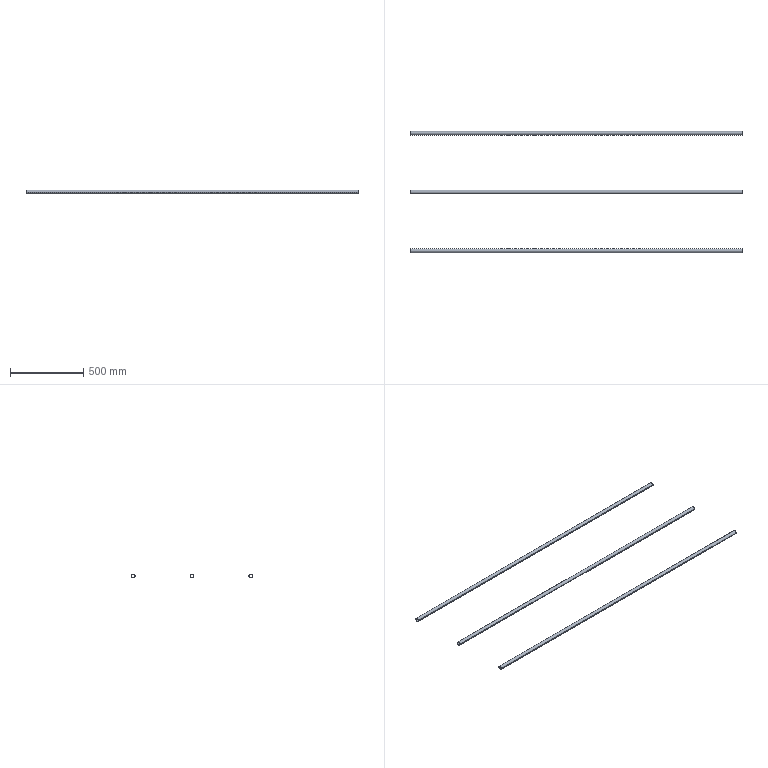Part | STEP file | E3-中转釜护栏8栏杆_Default<As Machined> | 3 solids | 18 faces | box 2260 x 825 x 25 mm | volume 750825 mm3 | cylinder 12 | plane 6 | commonest cylinder face diameters 22 x6 25 x6
STEP:
#1=CARTESIAN_POINT('',(0.,0.,0.));
#2=DIRECTION('',(0.,0.,1.));
#3=DIRECTION('',(1.,0.,0.));
#4=AXIS2_PLACEMENT_3D('',#1,#2,#3);
#5=CARTESIAN_POINT('',(1130.,787.5,0.));
#6=VERTEX_POINT('',#5);
#7=CARTESIAN_POINT('',(1130.,812.5,0.));
#8=VERTEX_POINT('',#7);
#9=CARTESIAN_POINT('',(1130.,800.,0.));
#10=DIRECTION('',(-1.,0.,0.));
#11=DIRECTION('',(0.,1.,0.));
#12=AXIS2_PLACEMENT_3D('',#9,#10,#11);
#13=CIRCLE('',#12,12.5);
#14=CARTESIAN_POINT('',(1130.,800.,0.));
#15=DIRECTION('',(-1.,0.,0.));
#16=DIRECTION('',(0.,-1.,0.));
#17=AXIS2_PLACEMENT_3D('',#14,#15,#16);
#18=CYLINDRICAL_SURFACE('',#17,12.5);
#19=CARTESIAN_POINT('',(-3.142,0.));
#20=DIRECTION('',(1.,0.));
#21=VECTOR('',#20,1.);
#22=LINE('',#19,#21);
#23=(GEOMETRIC_REPRESENTATION_CONTEXT(2)PARAMETRIC_REPRESENTATION_CONTEXT()REPRESENTATION_CONTEXT('',''));
#24=DEFINITIONAL_REPRESENTATION('',(#22),#23);
#25=PCURVE('',#18,#24);
#26=CARTESIAN_POINT('',(1130.,800.,0.));
#27=DIRECTION('',(1.,0.,0.));
#28=DIRECTION('',(0.,1.,0.));
#29=AXIS2_PLACEMENT_3D('',#26,#27,#28);
#30=PLANE('',#29);
#31=CARTESIAN_POINT('',(12.5,0.));
#32=CARTESIAN_POINT('',(12.5,-21.651));
#33=CARTESIAN_POINT('',(-6.25,-10.825));
#34=CARTESIAN_POINT('',(-25.,0.));
#35=CARTESIAN_POINT('',(-6.25,10.825));
#36=CARTESIAN_POINT('',(12.5,21.651));
#37=CARTESIAN_POINT('',(12.5,0.));
#38=(BOUNDED_CURVE()B_SPLINE_CURVE(2,(#31,#32,#33,#34,#35,#36,#37),.UNSPECIFIED.,.T.,.F.)B_SPLINE_CURVE_WITH_KNOTS((1,2,2,2,2,1),(-2.094,0.,2.094,4.189,6.283,8.378),.UNSPECIFIED.)CURVE()GEOMETRIC_REPRESENTATION_ITEM()RATIONAL_B_SPLINE_CURVE((1.,0.5,1.,0.5,1.,0.5,1.))REPRESENTATION_ITEM(''));
#39=(GEOMETRIC_REPRESENTATION_CONTEXT(2)PARAMETRIC_REPRESENTATION_CONTEXT()REPRESENTATION_CONTEXT('',''));
#40=DEFINITIONAL_REPRESENTATION('',(#38),#39);
#41=PCURVE('',#30,#40);
#42=SURFACE_CURVE('',#13,(#25,#41),.PCURVE_S1.);
#43=EDGE_CURVE('',#6,#8,#42,.T.);
#44=ORIENTED_EDGE('',*,*,#43,.T.);
#45=CARTESIAN_POINT('',(-1130.,812.5,0.));
#46=VERTEX_POINT('',#45);
#47=CARTESIAN_POINT('',(1130.,812.5,0.));
#48=DIRECTION('',(-1.,0.,0.));
#49=VECTOR('',#48,1.);
#50=LINE('',#47,#49);
#51=CARTESIAN_POINT('',(3.142,0.));
#52=DIRECTION('',(0.,1.));
#53=VECTOR('',#52,1.);
#54=LINE('',#51,#53);
#55=(GEOMETRIC_REPRESENTATION_CONTEXT(2)PARAMETRIC_REPRESENTATION_CONTEXT()REPRESENTATION_CONTEXT('',''));
#56=DEFINITIONAL_REPRESENTATION('',(#54),#55);
#57=PCURVE('',#18,#56);
#58=CARTESIAN_POINT('',(1130.,800.,0.));
#59=DIRECTION('',(-1.,0.,0.));
#60=DIRECTION('',(0.,-1.,0.));
#61=AXIS2_PLACEMENT_3D('',#58,#59,#60);
#62=CYLINDRICAL_SURFACE('',#61,12.5);
#63=CARTESIAN_POINT('',(3.142,0.));
#64=DIRECTION('',(0.,1.));
#65=VECTOR('',#64,1.);
#66=LINE('',#63,#65);
#67=(GEOMETRIC_REPRESENTATION_CONTEXT(2)PARAMETRIC_REPRESENTATION_CONTEXT()REPRESENTATION_CONTEXT('',''));
#68=DEFINITIONAL_REPRESENTATION('',(#66),#67);
#69=PCURVE('',#62,#68);
#70=SURFACE_CURVE('',#50,(#57,#69),.PCURVE_S1.);
#71=EDGE_CURVE('',#8,#46,#70,.T.);
#72=ORIENTED_EDGE('',*,*,#71,.T.);
#73=CARTESIAN_POINT('',(-1130.,787.5,0.));
#74=VERTEX_POINT('',#73);
#75=CARTESIAN_POINT('',(-1130.,800.,0.));
#76=DIRECTION('',(-1.,0.,0.));
#77=DIRECTION('',(0.,1.,0.));
#78=AXIS2_PLACEMENT_3D('',#75,#76,#77);
#79=CIRCLE('',#78,12.5);
#80=CARTESIAN_POINT('',(-3.142,2260.));
#81=DIRECTION('',(1.,0.));
#82=VECTOR('',#81,1.);
#83=LINE('',#80,#82);
#84=(GEOMETRIC_REPRESENTATION_CONTEXT(2)PARAMETRIC_REPRESENTATION_CONTEXT()REPRESENTATION_CONTEXT('',''));
#85=DEFINITIONAL_REPRESENTATION('',(#83),#84);
#86=PCURVE('',#18,#85);
#87=CARTESIAN_POINT('',(-1130.,800.,0.));
#88=DIRECTION('',(1.,0.,0.));
#89=DIRECTION('',(0.,1.,0.));
#90=AXIS2_PLACEMENT_3D('',#87,#88,#89);
#91=PLANE('',#90);
#92=CARTESIAN_POINT('',(12.5,0.));
#93=CARTESIAN_POINT('',(12.5,-21.651));
#94=CARTESIAN_POINT('',(-6.25,-10.825));
#95=CARTESIAN_POINT('',(-25.,0.));
#96=CARTESIAN_POINT('',(-6.25,10.825));
#97=CARTESIAN_POINT('',(12.5,21.651));
#98=CARTESIAN_POINT('',(12.5,0.));
#99=(BOUNDED_CURVE()B_SPLINE_CURVE(2,(#92,#93,#94,#95,#96,#97,#98),.UNSPECIFIED.,.T.,.F.)B_SPLINE_CURVE_WITH_KNOTS((1,2,2,2,2,1),(-2.094,0.,2.094,4.189,6.283,8.378),.UNSPECIFIED.)CURVE()GEOMETRIC_REPRESENTATION_ITEM()RATIONAL_B_SPLINE_CURVE((1.,0.5,1.,0.5,1.,0.5,1.))REPRESENTATION_ITEM(''));
#100=(GEOMETRIC_REPRESENTATION_CONTEXT(2)PARAMETRIC_REPRESENTATION_CONTEXT()REPRESENTATION_CONTEXT('',''));
#101=DEFINITIONAL_REPRESENTATION('',(#99),#100);
#102=PCURVE('',#91,#101);
#103=SURFACE_CURVE('',#79,(#86,#102),.PCURVE_S1.);
#104=EDGE_CURVE('',#74,#46,#103,.T.);
#105=ORIENTED_EDGE('',*,*,#104,.F.);
#106=CARTESIAN_POINT('',(1130.,787.5,0.));
#107=DIRECTION('',(-1.,0.,0.));
#108=VECTOR('',#107,1.);
#109=LINE('',#106,#108);
#110=CARTESIAN_POINT('',(0.,0.));
#111=DIRECTION('',(0.,1.));
#112=VECTOR('',#111,1.);
#113=LINE('',#110,#112);
#114=(GEOMETRIC_REPRESENTATION_CONTEXT(2)PARAMETRIC_REPRESENTATION_CONTEXT()REPRESENTATION_CONTEXT('',''));
#115=DEFINITIONAL_REPRESENTATION('',(#113),#114);
#116=PCURVE('',#18,#115);
#117=CARTESIAN_POINT('',(6.283,0.));
#118=DIRECTION('',(0.,1.));
#119=VECTOR('',#118,1.);
#120=LINE('',#117,#119);
#121=(GEOMETRIC_REPRESENTATION_CONTEXT(2)PARAMETRIC_REPRESENTATION_CONTEXT()REPRESENTATION_CONTEXT('',''));
#122=DEFINITIONAL_REPRESENTATION('',(#120),#121);
#123=PCURVE('',#62,#122);
#124=SURFACE_CURVE('',#109,(#116,#123),.PCURVE_S1.);
#125=EDGE_CURVE('',#6,#74,#124,.T.);
#126=ORIENTED_EDGE('',*,*,#125,.F.);
#127=EDGE_LOOP('',(#44,#72,#105,#126));
#128=FACE_BOUND('',#127,.T.);
#129=ADVANCED_FACE('',(#128),#18,.T.);
#130=CARTESIAN_POINT('',(1130.,789.,0.));
#131=VERTEX_POINT('',#130);
#132=CARTESIAN_POINT('',(-1130.,789.,0.));
#133=VERTEX_POINT('',#132);
#134=CARTESIAN_POINT('',(1130.,789.,0.));
#135=DIRECTION('',(-1.,0.,0.));
#136=VECTOR('',#135,1.);
#137=LINE('',#134,#136);
#138=CARTESIAN_POINT('',(1130.,800.,0.));
#139=DIRECTION('',(-1.,0.,0.));
#140=DIRECTION('',(0.,-1.,0.));
#141=AXIS2_PLACEMENT_3D('',#138,#139,#140);
#142=CYLINDRICAL_SURFACE('',#141,11.);
#143=CARTESIAN_POINT('',(6.283,0.));
#144=DIRECTION('',(0.,1.));
#145=VECTOR('',#144,1.);
#146=LINE('',#143,#145);
#147=(GEOMETRIC_REPRESENTATION_CONTEXT(2)PARAMETRIC_REPRESENTATION_CONTEXT()REPRESENTATION_CONTEXT('',''));
#148=DEFINITIONAL_REPRESENTATION('',(#146),#147);
#149=PCURVE('',#142,#148);
#150=CARTESIAN_POINT('',(1130.,800.,0.));
#151=DIRECTION('',(-1.,0.,0.));
#152=DIRECTION('',(0.,-1.,0.));
#153=AXIS2_PLACEMENT_3D('',#150,#151,#152);
#154=CYLINDRICAL_SURFACE('',#153,11.);
#155=CARTESIAN_POINT('',(0.,0.));
#156=DIRECTION('',(0.,1.));
#157=VECTOR('',#156,1.);
#158=LINE('',#155,#157);
#159=(GEOMETRIC_REPRESENTATION_CONTEXT(2)PARAMETRIC_REPRESENTATION_CONTEXT()REPRESENTATION_CONTEXT('',''));
#160=DEFINITIONAL_REPRESENTATION('',(#158),#159);
#161=PCURVE('',#154,#160);
#162=SURFACE_CURVE('',#137,(#149,#161),.PCURVE_S1.);
#163=EDGE_CURVE('',#131,#133,#162,.T.);
#164=ORIENTED_EDGE('',*,*,#163,.T.);
#165=CARTESIAN_POINT('',(-1130.,811.,0.));
#166=VERTEX_POINT('',#165);
#167=CARTESIAN_POINT('',(-1130.,800.,0.));
#168=DIRECTION('',(-1.,0.,0.));
#169=DIRECTION('',(0.,1.,0.));
#170=AXIS2_PLACEMENT_3D('',#167,#168,#169);
#171=CIRCLE('',#170,11.);
#172=CARTESIAN_POINT('',(3.142,2260.));
#173=DIRECTION('',(1.,0.));
#174=VECTOR('',#173,1.);
#175=LINE('',#172,#174);
#176=(GEOMETRIC_REPRESENTATION_CONTEXT(2)PARAMETRIC_REPRESENTATION_CONTEXT()REPRESENTATION_CONTEXT('',''));
#177=DEFINITIONAL_REPRESENTATION('',(#175),#176);
#178=PCURVE('',#142,#177);
#179=CARTESIAN_POINT('',(11.,0.));
#180=CARTESIAN_POINT('',(11.,-19.053));
#181=CARTESIAN_POINT('',(-5.5,-9.526));
#182=CARTESIAN_POINT('',(-22.,0.));
#183=CARTESIAN_POINT('',(-5.5,9.526));
#184=CARTESIAN_POINT('',(11.,19.053));
#185=CARTESIAN_POINT('',(11.,0.));
#186=(BOUNDED_CURVE()B_SPLINE_CURVE(2,(#179,#180,#181,#182,#183,#184,#185),.UNSPECIFIED.,.T.,.F.)B_SPLINE_CURVE_WITH_KNOTS((1,2,2,2,2,1),(-2.094,0.,2.094,4.189,6.283,8.378),.UNSPECIFIED.)CURVE()GEOMETRIC_REPRESENTATION_ITEM()RATIONAL_B_SPLINE_CURVE((1.,0.5,1.,0.5,1.,0.5,1.))REPRESENTATION_ITEM(''));
#187=(GEOMETRIC_REPRESENTATION_CONTEXT(2)PARAMETRIC_REPRESENTATION_CONTEXT()REPRESENTATION_CONTEXT('',''));
#188=DEFINITIONAL_REPRESENTATION('',(#186),#187);
#189=PCURVE('',#91,#188);
#190=SURFACE_CURVE('',#171,(#178,#189),.PCURVE_S1.);
#191=EDGE_CURVE('',#166,#133,#190,.T.);
#192=ORIENTED_EDGE('',*,*,#191,.F.);
#193=CARTESIAN_POINT('',(1130.,811.,0.));
#194=VERTEX_POINT('',#193);
#195=CARTESIAN_POINT('',(1130.,811.,0.));
#196=DIRECTION('',(-1.,0.,0.));
#197=VECTOR('',#196,1.);
#198=LINE('',#195,#197);
#199=CARTESIAN_POINT('',(3.142,0.));
#200=DIRECTION('',(0.,1.));
#201=VECTOR('',#200,1.);
#202=LINE('',#199,#201);
#203=(GEOMETRIC_REPRESENTATION_CONTEXT(2)PARAMETRIC_REPRESENTATION_CONTEXT()REPRESENTATION_CONTEXT('',''));
#204=DEFINITIONAL_REPRESENTATION('',(#202),#203);
#205=PCURVE('',#142,#204);
#206=CARTESIAN_POINT('',(3.142,0.));
#207=DIRECTION('',(0.,1.));
#208=VECTOR('',#207,1.);
#209=LINE('',#206,#208);
#210=(GEOMETRIC_REPRESENTATION_CONTEXT(2)PARAMETRIC_REPRESENTATION_CONTEXT()REPRESENTATION_CONTEXT('',''));
#211=DEFINITIONAL_REPRESENTATION('',(#209),#210);
#212=PCURVE('',#154,#211);
#213=SURFACE_CURVE('',#198,(#205,#212),.PCURVE_S1.);
#214=EDGE_CURVE('',#194,#166,#213,.T.);
#215=ORIENTED_EDGE('',*,*,#214,.F.);
#216=CARTESIAN_POINT('',(1130.,800.,0.));
#217=DIRECTION('',(-1.,0.,0.));
#218=DIRECTION('',(0.,1.,0.));
#219=AXIS2_PLACEMENT_3D('',#216,#217,#218);
#220=CIRCLE('',#219,11.);
#221=CARTESIAN_POINT('',(3.142,0.));
#222=DIRECTION('',(1.,0.));
#223=VECTOR('',#222,1.);
#224=LINE('',#221,#223);
#225=(GEOMETRIC_REPRESENTATION_CONTEXT(2)PARAMETRIC_REPRESENTATION_CONTEXT()REPRESENTATION_CONTEXT('',''));
#226=DEFINITIONAL_REPRESENTATION('',(#224),#225);
#227=PCURVE('',#142,#226);
#228=CARTESIAN_POINT('',(11.,0.));
#229=CARTESIAN_POINT('',(11.,-19.053));
#230=CARTESIAN_POINT('',(-5.5,-9.526));
#231=CARTESIAN_POINT('',(-22.,0.));
#232=CARTESIAN_POINT('',(-5.5,9.526));
#233=CARTESIAN_POINT('',(11.,19.053));
#234=CARTESIAN_POINT('',(11.,0.));
#235=(BOUNDED_CURVE()B_SPLINE_CURVE(2,(#228,#229,#230,#231,#232,#233,#234),.UNSPECIFIED.,.T.,.F.)B_SPLINE_CURVE_WITH_KNOTS((1,2,2,2,2,1),(-2.094,0.,2.094,4.189,6.283,8.378),.UNSPECIFIED.)CURVE()GEOMETRIC_REPRESENTATION_ITEM()RATIONAL_B_SPLINE_CURVE((1.,0.5,1.,0.5,1.,0.5,1.))REPRESENTATION_ITEM(''));
#236=(GEOMETRIC_REPRESENTATION_CONTEXT(2)PARAMETRIC_REPRESENTATION_CONTEXT()REPRESENTATION_CONTEXT('',''));
#237=DEFINITIONAL_REPRESENTATION('',(#235),#236);
#238=PCURVE('',#30,#237);
#239=SURFACE_CURVE('',#220,(#227,#238),.PCURVE_S1.);
#240=EDGE_CURVE('',#194,#131,#239,.T.);
#241=ORIENTED_EDGE('',*,*,#240,.T.);
#242=EDGE_LOOP('',(#164,#192,#215,#241));
#243=FACE_BOUND('',#242,.F.);
#244=ADVANCED_FACE('',(#243),#142,.F.);
#245=CARTESIAN_POINT('',(-1130.,800.,0.));
#246=DIRECTION('',(-1.,0.,0.));
#247=DIRECTION('',(0.,1.,0.));
#248=AXIS2_PLACEMENT_3D('',#245,#246,#247);
#249=CIRCLE('',#248,11.);
#250=CARTESIAN_POINT('',(-3.142,2260.));
#251=DIRECTION('',(1.,0.));
#252=VECTOR('',#251,1.);
#253=LINE('',#250,#252);
#254=(GEOMETRIC_REPRESENTATION_CONTEXT(2)PARAMETRIC_REPRESENTATION_CONTEXT()REPRESENTATION_CONTEXT('',''));
#255=DEFINITIONAL_REPRESENTATION('',(#253),#254);
#256=PCURVE('',#154,#255);
#257=CARTESIAN_POINT('',(11.,0.));
#258=CARTESIAN_POINT('',(11.,-19.053));
#259=CARTESIAN_POINT('',(-5.5,-9.526));
#260=CARTESIAN_POINT('',(-22.,0.));
#261=CARTESIAN_POINT('',(-5.5,9.526));
#262=CARTESIAN_POINT('',(11.,19.053));
#263=CARTESIAN_POINT('',(11.,0.));
#264=(BOUNDED_CURVE()B_SPLINE_CURVE(2,(#257,#258,#259,#260,#261,#262,#263),.UNSPECIFIED.,.T.,.F.)B_SPLINE_CURVE_WITH_KNOTS((1,2,2,2,2,1),(-2.094,0.,2.094,4.189,6.283,8.378),.UNSPECIFIED.)CURVE()GEOMETRIC_REPRESENTATION_ITEM()RATIONAL_B_SPLINE_CURVE((1.,0.5,1.,0.5,1.,0.5,1.))REPRESENTATION_ITEM(''));
#265=(GEOMETRIC_REPRESENTATION_CONTEXT(2)PARAMETRIC_REPRESENTATION_CONTEXT()REPRESENTATION_CONTEXT('',''));
#266=DEFINITIONAL_REPRESENTATION('',(#264),#265);
#267=PCURVE('',#91,#266);
#268=SURFACE_CURVE('',#249,(#256,#267),.PCURVE_S1.);
#269=EDGE_CURVE('',#133,#166,#268,.T.);
#270=ORIENTED_EDGE('',*,*,#269,.F.);
#271=ORIENTED_EDGE('',*,*,#163,.F.);
#272=CARTESIAN_POINT('',(1130.,800.,0.));
#273=DIRECTION('',(-1.,0.,0.));
#274=DIRECTION('',(0.,1.,0.));
#275=AXIS2_PLACEMENT_3D('',#272,#273,#274);
#276=CIRCLE('',#275,11.);
#277=CARTESIAN_POINT('',(-3.142,0.));
#278=DIRECTION('',(1.,0.));
#279=VECTOR('',#278,1.);
#280=LINE('',#277,#279);
#281=(GEOMETRIC_REPRESENTATION_CONTEXT(2)PARAMETRIC_REPRESENTATION_CONTEXT()REPRESENTATION_CONTEXT('',''));
#282=DEFINITIONAL_REPRESENTATION('',(#280),#281);
#283=PCURVE('',#154,#282);
#284=CARTESIAN_POINT('',(11.,0.));
#285=CARTESIAN_POINT('',(11.,-19.053));
#286=CARTESIAN_POINT('',(-5.5,-9.526));
#287=CARTESIAN_POINT('',(-22.,0.));
#288=CARTESIAN_POINT('',(-5.5,9.526));
#289=CARTESIAN_POINT('',(11.,19.053));
#290=CARTESIAN_POINT('',(11.,0.));
#291=(BOUNDED_CURVE()B_SPLINE_CURVE(2,(#284,#285,#286,#287,#288,#289,#290),.UNSPECIFIED.,.T.,.F.)B_SPLINE_CURVE_WITH_KNOTS((1,2,2,2,2,1),(-2.094,0.,2.094,4.189,6.283,8.378),.UNSPECIFIED.)CURVE()GEOMETRIC_REPRESENTATION_ITEM()RATIONAL_B_SPLINE_CURVE((1.,0.5,1.,0.5,1.,0.5,1.))REPRESENTATION_ITEM(''));
#292=(GEOMETRIC_REPRESENTATION_CONTEXT(2)PARAMETRIC_REPRESENTATION_CONTEXT()REPRESENTATION_CONTEXT('',''));
#293=DEFINITIONAL_REPRESENTATION('',(#291),#292);
#294=PCURVE('',#30,#293);
#295=SURFACE_CURVE('',#276,(#283,#294),.PCURVE_S1.);
#296=EDGE_CURVE('',#131,#194,#295,.T.);
#297=ORIENTED_EDGE('',*,*,#296,.T.);
#298=ORIENTED_EDGE('',*,*,#214,.T.);
#299=EDGE_LOOP('',(#270,#271,#297,#298));
#300=FACE_BOUND('',#299,.F.);
#301=ADVANCED_FACE('',(#300),#154,.F.);
#302=ORIENTED_EDGE('',*,*,#71,.F.);
#303=CARTESIAN_POINT('',(1130.,800.,0.));
#304=DIRECTION('',(-1.,0.,0.));
#305=DIRECTION('',(0.,1.,0.));
#306=AXIS2_PLACEMENT_3D('',#303,#304,#305);
#307=CIRCLE('',#306,12.5);
#308=CARTESIAN_POINT('',(3.142,0.));
#309=DIRECTION('',(1.,0.));
#310=VECTOR('',#309,1.);
#311=LINE('',#308,#310);
#312=(GEOMETRIC_REPRESENTATION_CONTEXT(2)PARAMETRIC_REPRESENTATION_CONTEXT()REPRESENTATION_CONTEXT('',''));
#313=DEFINITIONAL_REPRESENTATION('',(#311),#312);
#314=PCURVE('',#62,#313);
#315=CARTESIAN_POINT('',(12.5,0.));
#316=CARTESIAN_POINT('',(12.5,-21.651));
#317=CARTESIAN_POINT('',(-6.25,-10.825));
#318=CARTESIAN_POINT('',(-25.,0.));
#319=CARTESIAN_POINT('',(-6.25,10.825));
#320=CARTESIAN_POINT('',(12.5,21.651));
#321=CARTESIAN_POINT('',(12.5,0.));
#322=(BOUNDED_CURVE()B_SPLINE_CURVE(2,(#315,#316,#317,#318,#319,#320,#321),.UNSPECIFIED.,.T.,.F.)B_SPLINE_CURVE_WITH_KNOTS((1,2,2,2,2,1),(-2.094,0.,2.094,4.189,6.283,8.378),.UNSPECIFIED.)CURVE()GEOMETRIC_REPRESENTATION_ITEM()RATIONAL_B_SPLINE_CURVE((1.,0.5,1.,0.5,1.,0.5,1.))REPRESENTATION_ITEM(''));
#323=(GEOMETRIC_REPRESENTATION_CONTEXT(2)PARAMETRIC_REPRESENTATION_CONTEXT()REPRESENTATION_CONTEXT('',''));
#324=DEFINITIONAL_REPRESENTATION('',(#322),#323);
#325=PCURVE('',#30,#324);
#326=SURFACE_CURVE('',#307,(#314,#325),.PCURVE_S1.);
#327=EDGE_CURVE('',#8,#6,#326,.T.);
#328=ORIENTED_EDGE('',*,*,#327,.T.);
#329=ORIENTED_EDGE('',*,*,#125,.T.);
#330=CARTESIAN_POINT('',(-1130.,800.,0.));
#331=DIRECTION('',(-1.,0.,0.));
#332=DIRECTION('',(0.,1.,0.));
#333=AXIS2_PLACEMENT_3D('',#330,#331,#332);
#334=CIRCLE('',#333,12.5);
#335=CARTESIAN_POINT('',(3.142,2260.));
#336=DIRECTION('',(1.,0.));
#337=VECTOR('',#336,1.);
#338=LINE('',#335,#337);
#339=(GEOMETRIC_REPRESENTATION_CONTEXT(2)PARAMETRIC_REPRESENTATION_CONTEXT()REPRESENTATION_CONTEXT('',''));
#340=DEFINITIONAL_REPRESENTATION('',(#338),#339);
#341=PCURVE('',#62,#340);
#342=CARTESIAN_POINT('',(12.5,0.));
#343=CARTESIAN_POINT('',(12.5,-21.651));
#344=CARTESIAN_POINT('',(-6.25,-10.825));
#345=CARTESIAN_POINT('',(-25.,0.));
#346=CARTESIAN_POINT('',(-6.25,10.825));
#347=CARTESIAN_POINT('',(12.5,21.651));
#348=CARTESIAN_POINT('',(12.5,0.));
#349=(BOUNDED_CURVE()B_SPLINE_CURVE(2,(#342,#343,#344,#345,#346,#347,#348),.UNSPECIFIED.,.T.,.F.)B_SPLINE_CURVE_WITH_KNOTS((1,2,2,2,2,1),(-2.094,0.,2.094,4.189,6.283,8.378),.UNSPECIFIED.)CURVE()GEOMETRIC_REPRESENTATION_ITEM()RATIONAL_B_SPLINE_CURVE((1.,0.5,1.,0.5,1.,0.5,1.))REPRESENTATION_ITEM(''));
#350=(GEOMETRIC_REPRESENTATION_CONTEXT(2)PARAMETRIC_REPRESENTATION_CONTEXT()REPRESENTATION_CONTEXT('',''));
#351=DEFINITIONAL_REPRESENTATION('',(#349),#350);
#352=PCURVE('',#91,#351);
#353=SURFACE_CURVE('',#334,(#341,#352),.PCURVE_S1.);
#354=EDGE_CURVE('',#46,#74,#353,.T.);
#355=ORIENTED_EDGE('',*,*,#354,.F.);
#356=EDGE_LOOP('',(#302,#328,#329,#355));
#357=FACE_BOUND('',#356,.T.);
#358=ADVANCED_FACE('',(#357),#62,.T.);
#359=ORIENTED_EDGE('',*,*,#296,.T.);
#360=ORIENTED_EDGE('',*,*,#240,.T.);
#361=EDGE_LOOP('',(#359,#360));
#362=FACE_BOUND('',#361,.T.);
#363=ORIENTED_EDGE('',*,*,#43,.F.);
#364=ORIENTED_EDGE('',*,*,#327,.F.);
#365=EDGE_LOOP('',(#363,#364));
#366=FACE_BOUND('',#365,.T.);
#367=ADVANCED_FACE('',(#362,#366),#30,.T.);
#368=ORIENTED_EDGE('',*,*,#269,.F.);
#369=ORIENTED_EDGE('',*,*,#191,.F.);
#370=EDGE_LOOP('',(#368,#369));
#371=FACE_BOUND('',#370,.T.);
#372=ORIENTED_EDGE('',*,*,#104,.T.);
#373=ORIENTED_EDGE('',*,*,#354,.T.);
#374=EDGE_LOOP('',(#372,#373));
#375=FACE_BOUND('',#374,.T.);
#376=ADVANCED_FACE('',(#371,#375),#91,.F.);
#377=CLOSED_SHELL('',(#129,#244,#301,#358,#367,#376));
#378=MANIFOLD_SOLID_BREP('',#377);
#379=CARTESIAN_POINT('',(1130.,-12.5,0.));
#380=VERTEX_POINT('',#379);
#381=CARTESIAN_POINT('',(1130.,12.5,0.));
#382=VERTEX_POINT('',#381);
#383=CARTESIAN_POINT('',(1130.,0.,0.));
#384=DIRECTION('',(-1.,0.,0.));
#385=DIRECTION('',(0.,1.,0.));
#386=AXIS2_PLACEMENT_3D('',#383,#384,#385);
#387=CIRCLE('',#386,12.5);
#388=CARTESIAN_POINT('',(1130.,0.,0.));
#389=DIRECTION('',(-1.,0.,0.));
#390=DIRECTION('',(0.,-1.,0.));
#391=AXIS2_PLACEMENT_3D('',#388,#389,#390);
#392=CYLINDRICAL_SURFACE('',#391,12.5);
#393=CARTESIAN_POINT('',(-3.142,0.));
#394=DIRECTION('',(1.,0.));
#395=VECTOR('',#394,1.);
#396=LINE('',#393,#395);
#397=(GEOMETRIC_REPRESENTATION_CONTEXT(2)PARAMETRIC_REPRESENTATION_CONTEXT()REPRESENTATION_CONTEXT('',''));
#398=DEFINITIONAL_REPRESENTATION('',(#396),#397);
#399=PCURVE('',#392,#398);
#400=CARTESIAN_POINT('',(1130.,0.,0.));
#401=DIRECTION('',(1.,0.,0.));
#402=DIRECTION('',(0.,1.,0.));
#403=AXIS2_PLACEMENT_3D('',#400,#401,#402);
#404=PLANE('',#403);
#405=CARTESIAN_POINT('',(12.5,0.));
#406=CARTESIAN_POINT('',(12.5,-21.651));
#407=CARTESIAN_POINT('',(-6.25,-10.825));
#408=CARTESIAN_POINT('',(-25.,0.));
#409=CARTESIAN_POINT('',(-6.25,10.825));
#410=CARTESIAN_POINT('',(12.5,21.651));
#411=CARTESIAN_POINT('',(12.5,0.));
#412=(BOUNDED_CURVE()B_SPLINE_CURVE(2,(#405,#406,#407,#408,#409,#410,#411),.UNSPECIFIED.,.T.,.F.)B_SPLINE_CURVE_WITH_KNOTS((1,2,2,2,2,1),(-2.094,0.,2.094,4.189,6.283,8.378),.UNSPECIFIED.)CURVE()GEOMETRIC_REPRESENTATION_ITEM()RATIONAL_B_SPLINE_CURVE((1.,0.5,1.,0.5,1.,0.5,1.))REPRESENTATION_ITEM(''));
#413=(GEOMETRIC_REPRESENTATION_CONTEXT(2)PARAMETRIC_REPRESENTATION_CONTEXT()REPRESENTATION_CONTEXT('',''));
#414=DEFINITIONAL_REPRESENTATION('',(#412),#413);
#415=PCURVE('',#404,#414);
#416=SURFACE_CURVE('',#387,(#399,#415),.PCURVE_S1.);
#417=EDGE_CURVE('',#380,#382,#416,.T.);
#418=ORIENTED_EDGE('',*,*,#417,.T.);
#419=CARTESIAN_POINT('',(-1130.,12.5,0.));
#420=VERTEX_POINT('',#419);
#421=CARTESIAN_POINT('',(1130.,12.5,0.));
#422=DIRECTION('',(-1.,0.,0.));
#423=VECTOR('',#422,1.);
#424=LINE('',#421,#423);
#425=CARTESIAN_POINT('',(3.142,0.));
#426=DIRECTION('',(0.,1.));
#427=VECTOR('',#426,1.);
#428=LINE('',#425,#427);
#429=(GEOMETRIC_REPRESENTATION_CONTEXT(2)PARAMETRIC_REPRESENTATION_CONTEXT()REPRESENTATION_CONTEXT('',''));
#430=DEFINITIONAL_REPRESENTATION('',(#428),#429);
#431=PCURVE('',#392,#430);
#432=CARTESIAN_POINT('',(1130.,0.,0.));
#433=DIRECTION('',(-1.,0.,0.));
#434=DIRECTION('',(0.,-1.,0.));
#435=AXIS2_PLACEMENT_3D('',#432,#433,#434);
#436=CYLINDRICAL_SURFACE('',#435,12.5);
#437=CARTESIAN_POINT('',(3.142,0.));
#438=DIRECTION('',(0.,1.));
#439=VECTOR('',#438,1.);
#440=LINE('',#437,#439);
#441=(GEOMETRIC_REPRESENTATION_CONTEXT(2)PARAMETRIC_REPRESENTATION_CONTEXT()REPRESENTATION_CONTEXT('',''));
#442=DEFINITIONAL_REPRESENTATION('',(#440),#441);
#443=PCURVE('',#436,#442);
#444=SURFACE_CURVE('',#424,(#431,#443),.PCURVE_S1.);
#445=EDGE_CURVE('',#382,#420,#444,.T.);
#446=ORIENTED_EDGE('',*,*,#445,.T.);
#447=CARTESIAN_POINT('',(-1130.,-12.5,0.));
#448=VERTEX_POINT('',#447);
#449=CARTESIAN_POINT('',(-1130.,0.,0.));
#450=DIRECTION('',(-1.,0.,0.));
#451=DIRECTION('',(0.,1.,0.));
#452=AXIS2_PLACEMENT_3D('',#449,#450,#451);
#453=CIRCLE('',#452,12.5);
#454=CARTESIAN_POINT('',(-3.142,2260.));
#455=DIRECTION('',(1.,0.));
#456=VECTOR('',#455,1.);
#457=LINE('',#454,#456);
#458=(GEOMETRIC_REPRESENTATION_CONTEXT(2)PARAMETRIC_REPRESENTATION_CONTEXT()REPRESENTATION_CONTEXT('',''));
#459=DEFINITIONAL_REPRESENTATION('',(#457),#458);
#460=PCURVE('',#392,#459);
#461=CARTESIAN_POINT('',(-1130.,0.,0.));
#462=DIRECTION('',(1.,0.,0.));
#463=DIRECTION('',(0.,1.,0.));
#464=AXIS2_PLACEMENT_3D('',#461,#462,#463);
#465=PLANE('',#464);
#466=CARTESIAN_POINT('',(12.5,0.));
#467=CARTESIAN_POINT('',(12.5,-21.651));
#468=CARTESIAN_POINT('',(-6.25,-10.825));
#469=CARTESIAN_POINT('',(-25.,0.));
#470=CARTESIAN_POINT('',(-6.25,10.825));
#471=CARTESIAN_POINT('',(12.5,21.651));
#472=CARTESIAN_POINT('',(12.5,0.));
#473=(BOUNDED_CURVE()B_SPLINE_CURVE(2,(#466,#467,#468,#469,#470,#471,#472),.UNSPECIFIED.,.T.,.F.)B_SPLINE_CURVE_WITH_KNOTS((1,2,2,2,2,1),(-2.094,0.,2.094,4.189,6.283,8.378),.UNSPECIFIED.)CURVE()GEOMETRIC_REPRESENTATION_ITEM()RATIONAL_B_SPLINE_CURVE((1.,0.5,1.,0.5,1.,0.5,1.))REPRESENTATION_ITEM(''));
#474=(GEOMETRIC_REPRESENTATION_CONTEXT(2)PARAMETRIC_REPRESENTATION_CONTEXT()REPRESENTATION_CONTEXT('',''));
#475=DEFINITIONAL_REPRESENTATION('',(#473),#474);
#476=PCURVE('',#465,#475);
#477=SURFACE_CURVE('',#453,(#460,#476),.PCURVE_S1.);
#478=EDGE_CURVE('',#448,#420,#477,.T.);
#479=ORIENTED_EDGE('',*,*,#478,.F.);
#480=CARTESIAN_POINT('',(1130.,-12.5,0.));
#481=DIRECTION('',(-1.,0.,0.));
#482=VECTOR('',#481,1.);
#483=LINE('',#480,#482);
#484=CARTESIAN_POINT('',(0.,0.));
#485=DIRECTION('',(0.,1.));
#486=VECTOR('',#485,1.);
#487=LINE('',#484,#486);
#488=(GEOMETRIC_REPRESENTATION_CONTEXT(2)PARAMETRIC_REPRESENTATION_CONTEXT()REPRESENTATION_CONTEXT('',''));
#489=DEFINITIONAL_REPRESENTATION('',(#487),#488);
#490=PCURVE('',#392,#489);
#491=CARTESIAN_POINT('',(6.283,0.));
#492=DIRECTION('',(0.,1.));
#493=VECTOR('',#492,1.);
#494=LINE('',#491,#493);
#495=(GEOMETRIC_REPRESENTATION_CONTEXT(2)PARAMETRIC_REPRESENTATION_CONTEXT()REPRESENTATION_CONTEXT('',''));
#496=DEFINITIONAL_REPRESENTATION('',(#494),#495);
#497=PCURVE('',#436,#496);
#498=SURFACE_CURVE('',#483,(#490,#497),.PCURVE_S1.);
#499=EDGE_CURVE('',#380,#448,#498,.T.);
#500=ORIENTED_EDGE('',*,*,#499,.F.);
#501=EDGE_LOOP('',(#418,#446,#479,#500));
#502=FACE_BOUND('',#501,.T.);
#503=ADVANCED_FACE('',(#502),#392,.T.);
#504=CARTESIAN_POINT('',(1130.,-11.,0.));
#505=VERTEX_POINT('',#504);
#506=CARTESIAN_POINT('',(-1130.,-11.,0.));
#507=VERTEX_POINT('',#506);
#508=CARTESIAN_POINT('',(1130.,-11.,0.));
#509=DIRECTION('',(-1.,0.,0.));
#510=VECTOR('',#509,1.);
#511=LINE('',#508,#510);
#512=CARTESIAN_POINT('',(1130.,0.,0.));
#513=DIRECTION('',(-1.,0.,0.));
#514=DIRECTION('',(0.,-1.,0.));
#515=AXIS2_PLACEMENT_3D('',#512,#513,#514);
#516=CYLINDRICAL_SURFACE('',#515,11.);
#517=CARTESIAN_POINT('',(6.283,0.));
#518=DIRECTION('',(0.,1.));
#519=VECTOR('',#518,1.);
#520=LINE('',#517,#519);
#521=(GEOMETRIC_REPRESENTATION_CONTEXT(2)PARAMETRIC_REPRESENTATION_CONTEXT()REPRESENTATION_CONTEXT('',''));
#522=DEFINITIONAL_REPRESENTATION('',(#520),#521);
#523=PCURVE('',#516,#522);
#524=CARTESIAN_POINT('',(1130.,0.,0.));
#525=DIRECTION('',(-1.,0.,0.));
#526=DIRECTION('',(0.,-1.,0.));
#527=AXIS2_PLACEMENT_3D('',#524,#525,#526);
#528=CYLINDRICAL_SURFACE('',#527,11.);
#529=CARTESIAN_POINT('',(0.,0.));
#530=DIRECTION('',(0.,1.));
#531=VECTOR('',#530,1.);
#532=LINE('',#529,#531);
#533=(GEOMETRIC_REPRESENTATION_CONTEXT(2)PARAMETRIC_REPRESENTATION_CONTEXT()REPRESENTATION_CONTEXT('',''));
#534=DEFINITIONAL_REPRESENTATION('',(#532),#533);
#535=PCURVE('',#528,#534);
#536=SURFACE_CURVE('',#511,(#523,#535),.PCURVE_S1.);
#537=EDGE_CURVE('',#505,#507,#536,.T.);
#538=ORIENTED_EDGE('',*,*,#537,.T.);
#539=CARTESIAN_POINT('',(-1130.,11.,0.));
#540=VERTEX_POINT('',#539);
#541=CARTESIAN_POINT('',(-1130.,0.,0.));
#542=DIRECTION('',(-1.,0.,0.));
#543=DIRECTION('',(0.,1.,0.));
#544=AXIS2_PLACEMENT_3D('',#541,#542,#543);
#545=CIRCLE('',#544,11.);
#546=CARTESIAN_POINT('',(3.142,2260.));
#547=DIRECTION('',(1.,0.));
#548=VECTOR('',#547,1.);
#549=LINE('',#546,#548);
#550=(GEOMETRIC_REPRESENTATION_CONTEXT(2)PARAMETRIC_REPRESENTATION_CONTEXT()REPRESENTATION_CONTEXT('',''));
#551=DEFINITIONAL_REPRESENTATION('',(#549),#550);
#552=PCURVE('',#516,#551);
#553=CARTESIAN_POINT('',(11.,0.));
#554=CARTESIAN_POINT('',(11.,-19.053));
#555=CARTESIAN_POINT('',(-5.5,-9.526));
#556=CARTESIAN_POINT('',(-22.,0.));
#557=CARTESIAN_POINT('',(-5.5,9.526));
#558=CARTESIAN_POINT('',(11.,19.053));
#559=CARTESIAN_POINT('',(11.,0.));
#560=(BOUNDED_CURVE()B_SPLINE_CURVE(2,(#553,#554,#555,#556,#557,#558,#559),.UNSPECIFIED.,.T.,.F.)B_SPLINE_CURVE_WITH_KNOTS((1,2,2,2,2,1),(-2.094,0.,2.094,4.189,6.283,8.378),.UNSPECIFIED.)CURVE()GEOMETRIC_REPRESENTATION_ITEM()RATIONAL_B_SPLINE_CURVE((1.,0.5,1.,0.5,1.,0.5,1.))REPRESENTATION_ITEM(''));
#561=(GEOMETRIC_REPRESENTATION_CONTEXT(2)PARAMETRIC_REPRESENTATION_CONTEXT()REPRESENTATION_CONTEXT('',''));
#562=DEFINITIONAL_REPRESENTATION('',(#560),#561);
#563=PCURVE('',#465,#562);
#564=SURFACE_CURVE('',#545,(#552,#563),.PCURVE_S1.);
#565=EDGE_CURVE('',#540,#507,#564,.T.);
#566=ORIENTED_EDGE('',*,*,#565,.F.);
#567=CARTESIAN_POINT('',(1130.,11.,0.));
#568=VERTEX_POINT('',#567);
#569=CARTESIAN_POINT('',(1130.,11.,0.));
#570=DIRECTION('',(-1.,0.,0.));
#571=VECTOR('',#570,1.);
#572=LINE('',#569,#571);
#573=CARTESIAN_POINT('',(3.142,0.));
#574=DIRECTION('',(0.,1.));
#575=VECTOR('',#574,1.);
#576=LINE('',#573,#575);
#577=(GEOMETRIC_REPRESENTATION_CONTEXT(2)PARAMETRIC_REPRESENTATION_CONTEXT()REPRESENTATION_CONTEXT('',''));
#578=DEFINITIONAL_REPRESENTATION('',(#576),#577);
#579=PCURVE('',#516,#578);
#580=CARTESIAN_POINT('',(3.142,0.));
#581=DIRECTION('',(0.,1.));
#582=VECTOR('',#581,1.);
#583=LINE('',#580,#582);
#584=(GEOMETRIC_REPRESENTATION_CONTEXT(2)PARAMETRIC_REPRESENTATION_CONTEXT()REPRESENTATION_CONTEXT('',''));
#585=DEFINITIONAL_REPRESENTATION('',(#583),#584);
#586=PCURVE('',#528,#585);
#587=SURFACE_CURVE('',#572,(#579,#586),.PCURVE_S1.);
#588=EDGE_CURVE('',#568,#540,#587,.T.);
#589=ORIENTED_EDGE('',*,*,#588,.F.);
#590=CARTESIAN_POINT('',(1130.,0.,0.));
#591=DIRECTION('',(-1.,0.,0.));
#592=DIRECTION('',(0.,1.,0.));
#593=AXIS2_PLACEMENT_3D('',#590,#591,#592);
#594=CIRCLE('',#593,11.);
#595=CARTESIAN_POINT('',(3.142,0.));
#596=DIRECTION('',(1.,0.));
#597=VECTOR('',#596,1.);
#598=LINE('',#595,#597);
#599=(GEOMETRIC_REPRESENTATION_CONTEXT(2)PARAMETRIC_REPRESENTATION_CONTEXT()REPRESENTATION_CONTEXT('',''));
#600=DEFINITIONAL_REPRESENTATION('',(#598),#599);
#601=PCURVE('',#516,#600);
#602=CARTESIAN_POINT('',(11.,0.));
#603=CARTESIAN_POINT('',(11.,-19.053));
#604=CARTESIAN_POINT('',(-5.5,-9.526));
#605=CARTESIAN_POINT('',(-22.,0.));
#606=CARTESIAN_POINT('',(-5.5,9.526));
#607=CARTESIAN_POINT('',(11.,19.053));
#608=CARTESIAN_POINT('',(11.,0.));
#609=(BOUNDED_CURVE()B_SPLINE_CURVE(2,(#602,#603,#604,#605,#606,#607,#608),.UNSPECIFIED.,.T.,.F.)B_SPLINE_CURVE_WITH_KNOTS((1,2,2,2,2,1),(-2.094,0.,2.094,4.189,6.283,8.378),.UNSPECIFIED.)CURVE()GEOMETRIC_REPRESENTATION_ITEM()RATIONAL_B_SPLINE_CURVE((1.,0.5,1.,0.5,1.,0.5,1.))REPRESENTATION_ITEM(''));
#610=(GEOMETRIC_REPRESENTATION_CONTEXT(2)PARAMETRIC_REPRESENTATION_CONTEXT()REPRESENTATION_CONTEXT('',''));
#611=DEFINITIONAL_REPRESENTATION('',(#609),#610);
#612=PCURVE('',#404,#611);
#613=SURFACE_CURVE('',#594,(#601,#612),.PCURVE_S1.);
#614=EDGE_CURVE('',#568,#505,#613,.T.);
#615=ORIENTED_EDGE('',*,*,#614,.T.);
#616=EDGE_LOOP('',(#538,#566,#589,#615));
#617=FACE_BOUND('',#616,.F.);
#618=ADVANCED_FACE('',(#617),#516,.F.);
#619=CARTESIAN_POINT('',(-1130.,0.,0.));
#620=DIRECTION('',(-1.,0.,0.));
#621=DIRECTION('',(0.,1.,0.));
#622=AXIS2_PLACEMENT_3D('',#619,#620,#621);
#623=CIRCLE('',#622,11.);
#624=CARTESIAN_POINT('',(-3.142,2260.));
#625=DIRECTION('',(1.,0.));
#626=VECTOR('',#625,1.);
#627=LINE('',#624,#626);
#628=(GEOMETRIC_REPRESENTATION_CONTEXT(2)PARAMETRIC_REPRESENTATION_CONTEXT()REPRESENTATION_CONTEXT('',''));
#629=DEFINITIONAL_REPRESENTATION('',(#627),#628);
#630=PCURVE('',#528,#629);
#631=CARTESIAN_POINT('',(11.,0.));
#632=CARTESIAN_POINT('',(11.,-19.053));
#633=CARTESIAN_POINT('',(-5.5,-9.526));
#634=CARTESIAN_POINT('',(-22.,0.));
#635=CARTESIAN_POINT('',(-5.5,9.526));
#636=CARTESIAN_POINT('',(11.,19.053));
#637=CARTESIAN_POINT('',(11.,0.));
#638=(BOUNDED_CURVE()B_SPLINE_CURVE(2,(#631,#632,#633,#634,#635,#636,#637),.UNSPECIFIED.,.T.,.F.)B_SPLINE_CURVE_WITH_KNOTS((1,2,2,2,2,1),(-2.094,0.,2.094,4.189,6.283,8.378),.UNSPECIFIED.)CURVE()GEOMETRIC_REPRESENTATION_ITEM()RATIONAL_B_SPLINE_CURVE((1.,0.5,1.,0.5,1.,0.5,1.))REPRESENTATION_ITEM(''));
#639=(GEOMETRIC_REPRESENTATION_CONTEXT(2)PARAMETRIC_REPRESENTATION_CONTEXT()REPRESENTATION_CONTEXT('',''));
#640=DEFINITIONAL_REPRESENTATION('',(#638),#639);
#641=PCURVE('',#465,#640);
#642=SURFACE_CURVE('',#623,(#630,#641),.PCURVE_S1.);
#643=EDGE_CURVE('',#507,#540,#642,.T.);
#644=ORIENTED_EDGE('',*,*,#643,.F.);
#645=ORIENTED_EDGE('',*,*,#537,.F.);
#646=CARTESIAN_POINT('',(1130.,0.,0.));
#647=DIRECTION('',(-1.,0.,0.));
#648=DIRECTION('',(0.,1.,0.));
#649=AXIS2_PLACEMENT_3D('',#646,#647,#648);
#650=CIRCLE('',#649,11.);
#651=CARTESIAN_POINT('',(-3.142,0.));
#652=DIRECTION('',(1.,0.));
#653=VECTOR('',#652,1.);
#654=LINE('',#651,#653);
#655=(GEOMETRIC_REPRESENTATION_CONTEXT(2)PARAMETRIC_REPRESENTATION_CONTEXT()REPRESENTATION_CONTEXT('',''));
#656=DEFINITIONAL_REPRESENTATION('',(#654),#655);
#657=PCURVE('',#528,#656);
#658=CARTESIAN_POINT('',(11.,0.));
#659=CARTESIAN_POINT('',(11.,-19.053));
#660=CARTESIAN_POINT('',(-5.5,-9.526));
#661=CARTESIAN_POINT('',(-22.,0.));
#662=CARTESIAN_POINT('',(-5.5,9.526));
#663=CARTESIAN_POINT('',(11.,19.053));
#664=CARTESIAN_POINT('',(11.,0.));
#665=(BOUNDED_CURVE()B_SPLINE_CURVE(2,(#658,#659,#660,#661,#662,#663,#664),.UNSPECIFIED.,.T.,.F.)B_SPLINE_CURVE_WITH_KNOTS((1,2,2,2,2,1),(-2.094,0.,2.094,4.189,6.283,8.378),.UNSPECIFIED.)CURVE()GEOMETRIC_REPRESENTATION_ITEM()RATIONAL_B_SPLINE_CURVE((1.,0.5,1.,0.5,1.,0.5,1.))REPRESENTATION_ITEM(''));
#666=(GEOMETRIC_REPRESENTATION_CONTEXT(2)PARAMETRIC_REPRESENTATION_CONTEXT()REPRESENTATION_CONTEXT('',''));
#667=DEFINITIONAL_REPRESENTATION('',(#665),#666);
#668=PCURVE('',#404,#667);
#669=SURFACE_CURVE('',#650,(#657,#668),.PCURVE_S1.);
#670=EDGE_CURVE('',#505,#568,#669,.T.);
#671=ORIENTED_EDGE('',*,*,#670,.T.);
#672=ORIENTED_EDGE('',*,*,#588,.T.);
#673=EDGE_LOOP('',(#644,#645,#671,#672));
#674=FACE_BOUND('',#673,.F.);
#675=ADVANCED_FACE('',(#674),#528,.F.);
#676=ORIENTED_EDGE('',*,*,#445,.F.);
#677=CARTESIAN_POINT('',(1130.,0.,0.));
#678=DIRECTION('',(-1.,0.,0.));
#679=DIRECTION('',(0.,1.,0.));
#680=AXIS2_PLACEMENT_3D('',#677,#678,#679);
#681=CIRCLE('',#680,12.5);
#682=CARTESIAN_POINT('',(3.142,0.));
#683=DIRECTION('',(1.,0.));
#684=VECTOR('',#683,1.);
#685=LINE('',#682,#684);
#686=(GEOMETRIC_REPRESENTATION_CONTEXT(2)PARAMETRIC_REPRESENTATION_CONTEXT()REPRESENTATION_CONTEXT('',''));
#687=DEFINITIONAL_REPRESENTATION('',(#685),#686);
#688=PCURVE('',#436,#687);
#689=CARTESIAN_POINT('',(12.5,0.));
#690=CARTESIAN_POINT('',(12.5,-21.651));
#691=CARTESIAN_POINT('',(-6.25,-10.825));
#692=CARTESIAN_POINT('',(-25.,0.));
#693=CARTESIAN_POINT('',(-6.25,10.825));
#694=CARTESIAN_POINT('',(12.5,21.651));
#695=CARTESIAN_POINT('',(12.5,0.));
#696=(BOUNDED_CURVE()B_SPLINE_CURVE(2,(#689,#690,#691,#692,#693,#694,#695),.UNSPECIFIED.,.T.,.F.)B_SPLINE_CURVE_WITH_KNOTS((1,2,2,2,2,1),(-2.094,0.,2.094,4.189,6.283,8.378),.UNSPECIFIED.)CURVE()GEOMETRIC_REPRESENTATION_ITEM()RATIONAL_B_SPLINE_CURVE((1.,0.5,1.,0.5,1.,0.5,1.))REPRESENTATION_ITEM(''));
#697=(GEOMETRIC_REPRESENTATION_CONTEXT(2)PARAMETRIC_REPRESENTATION_CONTEXT()REPRESENTATION_CONTEXT('',''));
#698=DEFINITIONAL_REPRESENTATION('',(#696),#697);
#699=PCURVE('',#404,#698);
#700=SURFACE_CURVE('',#681,(#688,#699),.PCURVE_S1.);
#701=EDGE_CURVE('',#382,#380,#700,.T.);
#702=ORIENTED_EDGE('',*,*,#701,.T.);
#703=ORIENTED_EDGE('',*,*,#499,.T.);
#704=CARTESIAN_POINT('',(-1130.,0.,0.));
#705=DIRECTION('',(-1.,0.,0.));
#706=DIRECTION('',(0.,1.,0.));
#707=AXIS2_PLACEMENT_3D('',#704,#705,#706);
#708=CIRCLE('',#707,12.5);
#709=CARTESIAN_POINT('',(3.142,2260.));
#710=DIRECTION('',(1.,0.));
#711=VECTOR('',#710,1.);
#712=LINE('',#709,#711);
#713=(GEOMETRIC_REPRESENTATION_CONTEXT(2)PARAMETRIC_REPRESENTATION_CONTEXT()REPRESENTATION_CONTEXT('',''));
#714=DEFINITIONAL_REPRESENTATION('',(#712),#713);
#715=PCURVE('',#436,#714);
#716=CARTESIAN_POINT('',(12.5,0.));
#717=CARTESIAN_POINT('',(12.5,-21.651));
#718=CARTESIAN_POINT('',(-6.25,-10.825));
#719=CARTESIAN_POINT('',(-25.,0.));
#720=CARTESIAN_POINT('',(-6.25,10.825));
#721=CARTESIAN_POINT('',(12.5,21.651));
#722=CARTESIAN_POINT('',(12.5,0.));
#723=(BOUNDED_CURVE()B_SPLINE_CURVE(2,(#716,#717,#718,#719,#720,#721,#722),.UNSPECIFIED.,.T.,.F.)B_SPLINE_CURVE_WITH_KNOTS((1,2,2,2,2,1),(-2.094,0.,2.094,4.189,6.283,8.378),.UNSPECIFIED.)CURVE()GEOMETRIC_REPRESENTATION_ITEM()RATIONAL_B_SPLINE_CURVE((1.,0.5,1.,0.5,1.,0.5,1.))REPRESENTATION_ITEM(''));
#724=(GEOMETRIC_REPRESENTATION_CONTEXT(2)PARAMETRIC_REPRESENTATION_CONTEXT()REPRESENTATION_CONTEXT('',''));
#725=DEFINITIONAL_REPRESENTATION('',(#723),#724);
#726=PCURVE('',#465,#725);
#727=SURFACE_CURVE('',#708,(#715,#726),.PCURVE_S1.);
#728=EDGE_CURVE('',#420,#448,#727,.T.);
#729=ORIENTED_EDGE('',*,*,#728,.F.);
#730=EDGE_LOOP('',(#676,#702,#703,#729));
#731=FACE_BOUND('',#730,.T.);
#732=ADVANCED_FACE('',(#731),#436,.T.);
#733=ORIENTED_EDGE('',*,*,#670,.T.);
#734=ORIENTED_EDGE('',*,*,#614,.T.);
#735=EDGE_LOOP('',(#733,#734));
#736=FACE_BOUND('',#735,.T.);
#737=ORIENTED_EDGE('',*,*,#417,.F.);
#738=ORIENTED_EDGE('',*,*,#701,.F.);
#739=EDGE_LOOP('',(#737,#738));
#740=FACE_BOUND('',#739,.T.);
#741=ADVANCED_FACE('',(#736,#740),#404,.T.);
#742=ORIENTED_EDGE('',*,*,#643,.F.);
#743=ORIENTED_EDGE('',*,*,#565,.F.);
#744=EDGE_LOOP('',(#742,#743));
#745=FACE_BOUND('',#744,.T.);
#746=ORIENTED_EDGE('',*,*,#478,.T.);
#747=ORIENTED_EDGE('',*,*,#728,.T.);
#748=EDGE_LOOP('',(#746,#747));
#749=FACE_BOUND('',#748,.T.);
#750=ADVANCED_FACE('',(#745,#749),#465,.F.);
#751=CLOSED_SHELL('',(#503,#618,#675,#732,#741,#750));
#752=MANIFOLD_SOLID_BREP('',#751);
#753=CARTESIAN_POINT('',(1130.,387.5,0.));
#754=VERTEX_POINT('',#753);
#755=CARTESIAN_POINT('',(1130.,412.5,0.));
#756=VERTEX_POINT('',#755);
#757=CARTESIAN_POINT('',(1130.,400.,0.));
#758=DIRECTION('',(-1.,0.,0.));
#759=DIRECTION('',(0.,1.,0.));
#760=AXIS2_PLACEMENT_3D('',#757,#758,#759);
#761=CIRCLE('',#760,12.5);
#762=CARTESIAN_POINT('',(1130.,400.,0.));
#763=DIRECTION('',(-1.,0.,0.));
#764=DIRECTION('',(0.,-1.,0.));
#765=AXIS2_PLACEMENT_3D('',#762,#763,#764);
#766=CYLINDRICAL_SURFACE('',#765,12.5);
#767=CARTESIAN_POINT('',(-3.142,0.));
#768=DIRECTION('',(1.,0.));
#769=VECTOR('',#768,1.);
#770=LINE('',#767,#769);
#771=(GEOMETRIC_REPRESENTATION_CONTEXT(2)PARAMETRIC_REPRESENTATION_CONTEXT()REPRESENTATION_CONTEXT('',''));
#772=DEFINITIONAL_REPRESENTATION('',(#770),#771);
#773=PCURVE('',#766,#772);
#774=CARTESIAN_POINT('',(1130.,400.,0.));
#775=DIRECTION('',(1.,0.,0.));
#776=DIRECTION('',(0.,1.,0.));
#777=AXIS2_PLACEMENT_3D('',#774,#775,#776);
#778=PLANE('',#777);
#779=CARTESIAN_POINT('',(12.5,0.));
#780=CARTESIAN_POINT('',(12.5,-21.651));
#781=CARTESIAN_POINT('',(-6.25,-10.825));
#782=CARTESIAN_POINT('',(-25.,0.));
#783=CARTESIAN_POINT('',(-6.25,10.825));
#784=CARTESIAN_POINT('',(12.5,21.651));
#785=CARTESIAN_POINT('',(12.5,0.));
#786=(BOUNDED_CURVE()B_SPLINE_CURVE(2,(#779,#780,#781,#782,#783,#784,#785),.UNSPECIFIED.,.T.,.F.)B_SPLINE_CURVE_WITH_KNOTS((1,2,2,2,2,1),(-2.094,0.,2.094,4.189,6.283,8.378),.UNSPECIFIED.)CURVE()GEOMETRIC_REPRESENTATION_ITEM()RATIONAL_B_SPLINE_CURVE((1.,0.5,1.,0.5,1.,0.5,1.))REPRESENTATION_ITEM(''));
#787=(GEOMETRIC_REPRESENTATION_CONTEXT(2)PARAMETRIC_REPRESENTATION_CONTEXT()REPRESENTATION_CONTEXT('',''));
#788=DEFINITIONAL_REPRESENTATION('',(#786),#787);
#789=PCURVE('',#778,#788);
#790=SURFACE_CURVE('',#761,(#773,#789),.PCURVE_S1.);
#791=EDGE_CURVE('',#754,#756,#790,.T.);
#792=ORIENTED_EDGE('',*,*,#791,.T.);
#793=CARTESIAN_POINT('',(-1130.,412.5,0.));
#794=VERTEX_POINT('',#793);
#795=CARTESIAN_POINT('',(1130.,412.5,0.));
#796=DIRECTION('',(-1.,0.,0.));
#797=VECTOR('',#796,1.);
#798=LINE('',#795,#797);
#799=CARTESIAN_POINT('',(3.142,0.));
#800=DIRECTION('',(0.,1.));
#801=VECTOR('',#800,1.);
#802=LINE('',#799,#801);
#803=(GEOMETRIC_REPRESENTATION_CONTEXT(2)PARAMETRIC_REPRESENTATION_CONTEXT()REPRESENTATION_CONTEXT('',''));
#804=DEFINITIONAL_REPRESENTATION('',(#802),#803);
#805=PCURVE('',#766,#804);
#806=CARTESIAN_POINT('',(1130.,400.,0.));
#807=DIRECTION('',(-1.,0.,0.));
#808=DIRECTION('',(0.,-1.,0.));
#809=AXIS2_PLACEMENT_3D('',#806,#807,#808);
#810=CYLINDRICAL_SURFACE('',#809,12.5);
#811=CARTESIAN_POINT('',(3.142,0.));
#812=DIRECTION('',(0.,1.));
#813=VECTOR('',#812,1.);
#814=LINE('',#811,#813);
#815=(GEOMETRIC_REPRESENTATION_CONTEXT(2)PARAMETRIC_REPRESENTATION_CONTEXT()REPRESENTATION_CONTEXT('',''));
#816=DEFINITIONAL_REPRESENTATION('',(#814),#815);
#817=PCURVE('',#810,#816);
#818=SURFACE_CURVE('',#798,(#805,#817),.PCURVE_S1.);
#819=EDGE_CURVE('',#756,#794,#818,.T.);
#820=ORIENTED_EDGE('',*,*,#819,.T.);
#821=CARTESIAN_POINT('',(-1130.,387.5,0.));
#822=VERTEX_POINT('',#821);
#823=CARTESIAN_POINT('',(-1130.,400.,0.));
#824=DIRECTION('',(-1.,0.,0.));
#825=DIRECTION('',(0.,1.,0.));
#826=AXIS2_PLACEMENT_3D('',#823,#824,#825);
#827=CIRCLE('',#826,12.5);
#828=CARTESIAN_POINT('',(-3.142,2260.));
#829=DIRECTION('',(1.,0.));
#830=VECTOR('',#829,1.);
#831=LINE('',#828,#830);
#832=(GEOMETRIC_REPRESENTATION_CONTEXT(2)PARAMETRIC_REPRESENTATION_CONTEXT()REPRESENTATION_CONTEXT('',''));
#833=DEFINITIONAL_REPRESENTATION('',(#831),#832);
#834=PCURVE('',#766,#833);
#835=CARTESIAN_POINT('',(-1130.,400.,0.));
#836=DIRECTION('',(1.,0.,0.));
#837=DIRECTION('',(0.,1.,0.));
#838=AXIS2_PLACEMENT_3D('',#835,#836,#837);
#839=PLANE('',#838);
#840=CARTESIAN_POINT('',(12.5,0.));
#841=CARTESIAN_POINT('',(12.5,-21.651));
#842=CARTESIAN_POINT('',(-6.25,-10.825));
#843=CARTESIAN_POINT('',(-25.,0.));
#844=CARTESIAN_POINT('',(-6.25,10.825));
#845=CARTESIAN_POINT('',(12.5,21.651));
#846=CARTESIAN_POINT('',(12.5,0.));
#847=(BOUNDED_CURVE()B_SPLINE_CURVE(2,(#840,#841,#842,#843,#844,#845,#846),.UNSPECIFIED.,.T.,.F.)B_SPLINE_CURVE_WITH_KNOTS((1,2,2,2,2,1),(-2.094,0.,2.094,4.189,6.283,8.378),.UNSPECIFIED.)CURVE()GEOMETRIC_REPRESENTATION_ITEM()RATIONAL_B_SPLINE_CURVE((1.,0.5,1.,0.5,1.,0.5,1.))REPRESENTATION_ITEM(''));
#848=(GEOMETRIC_REPRESENTATION_CONTEXT(2)PARAMETRIC_REPRESENTATION_CONTEXT()REPRESENTATION_CONTEXT('',''));
#849=DEFINITIONAL_REPRESENTATION('',(#847),#848);
#850=PCURVE('',#839,#849);
#851=SURFACE_CURVE('',#827,(#834,#850),.PCURVE_S1.);
#852=EDGE_CURVE('',#822,#794,#851,.T.);
#853=ORIENTED_EDGE('',*,*,#852,.F.);
#854=CARTESIAN_POINT('',(1130.,387.5,0.));
#855=DIRECTION('',(-1.,0.,0.));
#856=VECTOR('',#855,1.);
#857=LINE('',#854,#856);
#858=CARTESIAN_POINT('',(0.,0.));
#859=DIRECTION('',(0.,1.));
#860=VECTOR('',#859,1.);
#861=LINE('',#858,#860);
#862=(GEOMETRIC_REPRESENTATION_CONTEXT(2)PARAMETRIC_REPRESENTATION_CONTEXT()REPRESENTATION_CONTEXT('',''));
#863=DEFINITIONAL_REPRESENTATION('',(#861),#862);
#864=PCURVE('',#766,#863);
#865=CARTESIAN_POINT('',(6.283,0.));
#866=DIRECTION('',(0.,1.));
#867=VECTOR('',#866,1.);
#868=LINE('',#865,#867);
#869=(GEOMETRIC_REPRESENTATION_CONTEXT(2)PARAMETRIC_REPRESENTATION_CONTEXT()REPRESENTATION_CONTEXT('',''));
#870=DEFINITIONAL_REPRESENTATION('',(#868),#869);
#871=PCURVE('',#810,#870);
#872=SURFACE_CURVE('',#857,(#864,#871),.PCURVE_S1.);
#873=EDGE_CURVE('',#754,#822,#872,.T.);
#874=ORIENTED_EDGE('',*,*,#873,.F.);
#875=EDGE_LOOP('',(#792,#820,#853,#874));
#876=FACE_BOUND('',#875,.T.);
#877=ADVANCED_FACE('',(#876),#766,.T.);
#878=CARTESIAN_POINT('',(1130.,389.,0.));
#879=VERTEX_POINT('',#878);
#880=CARTESIAN_POINT('',(-1130.,389.,0.));
#881=VERTEX_POINT('',#880);
#882=CARTESIAN_POINT('',(1130.,389.,0.));
#883=DIRECTION('',(-1.,0.,0.));
#884=VECTOR('',#883,1.);
#885=LINE('',#882,#884);
#886=CARTESIAN_POINT('',(1130.,400.,0.));
#887=DIRECTION('',(-1.,0.,0.));
#888=DIRECTION('',(0.,-1.,0.));
#889=AXIS2_PLACEMENT_3D('',#886,#887,#888);
#890=CYLINDRICAL_SURFACE('',#889,11.);
#891=CARTESIAN_POINT('',(6.283,0.));
#892=DIRECTION('',(0.,1.));
#893=VECTOR('',#892,1.);
#894=LINE('',#891,#893);
#895=(GEOMETRIC_REPRESENTATION_CONTEXT(2)PARAMETRIC_REPRESENTATION_CONTEXT()REPRESENTATION_CONTEXT('',''));
#896=DEFINITIONAL_REPRESENTATION('',(#894),#895);
#897=PCURVE('',#890,#896);
#898=CARTESIAN_POINT('',(1130.,400.,0.));
#899=DIRECTION('',(-1.,0.,0.));
#900=DIRECTION('',(0.,-1.,0.));
#901=AXIS2_PLACEMENT_3D('',#898,#899,#900);
#902=CYLINDRICAL_SURFACE('',#901,11.);
#903=CARTESIAN_POINT('',(0.,0.));
#904=DIRECTION('',(0.,1.));
#905=VECTOR('',#904,1.);
#906=LINE('',#903,#905);
#907=(GEOMETRIC_REPRESENTATION_CONTEXT(2)PARAMETRIC_REPRESENTATION_CONTEXT()REPRESENTATION_CONTEXT('',''));
#908=DEFINITIONAL_REPRESENTATION('',(#906),#907);
#909=PCURVE('',#902,#908);
#910=SURFACE_CURVE('',#885,(#897,#909),.PCURVE_S1.);
#911=EDGE_CURVE('',#879,#881,#910,.T.);
#912=ORIENTED_EDGE('',*,*,#911,.T.);
#913=CARTESIAN_POINT('',(-1130.,411.,0.));
#914=VERTEX_POINT('',#913);
#915=CARTESIAN_POINT('',(-1130.,400.,0.));
#916=DIRECTION('',(-1.,0.,0.));
#917=DIRECTION('',(0.,1.,0.));
#918=AXIS2_PLACEMENT_3D('',#915,#916,#917);
#919=CIRCLE('',#918,11.);
#920=CARTESIAN_POINT('',(3.142,2260.));
#921=DIRECTION('',(1.,0.));
#922=VECTOR('',#921,1.);
#923=LINE('',#920,#922);
#924=(GEOMETRIC_REPRESENTATION_CONTEXT(2)PARAMETRIC_REPRESENTATION_CONTEXT()REPRESENTATION_CONTEXT('',''));
#925=DEFINITIONAL_REPRESENTATION('',(#923),#924);
#926=PCURVE('',#890,#925);
#927=CARTESIAN_POINT('',(11.,0.));
#928=CARTESIAN_POINT('',(11.,-19.053));
#929=CARTESIAN_POINT('',(-5.5,-9.526));
#930=CARTESIAN_POINT('',(-22.,0.));
#931=CARTESIAN_POINT('',(-5.5,9.526));
#932=CARTESIAN_POINT('',(11.,19.053));
#933=CARTESIAN_POINT('',(11.,0.));
#934=(BOUNDED_CURVE()B_SPLINE_CURVE(2,(#927,#928,#929,#930,#931,#932,#933),.UNSPECIFIED.,.T.,.F.)B_SPLINE_CURVE_WITH_KNOTS((1,2,2,2,2,1),(-2.094,0.,2.094,4.189,6.283,8.378),.UNSPECIFIED.)CURVE()GEOMETRIC_REPRESENTATION_ITEM()RATIONAL_B_SPLINE_CURVE((1.,0.5,1.,0.5,1.,0.5,1.))REPRESENTATION_ITEM(''));
#935=(GEOMETRIC_REPRESENTATION_CONTEXT(2)PARAMETRIC_REPRESENTATION_CONTEXT()REPRESENTATION_CONTEXT('',''));
#936=DEFINITIONAL_REPRESENTATION('',(#934),#935);
#937=PCURVE('',#839,#936);
#938=SURFACE_CURVE('',#919,(#926,#937),.PCURVE_S1.);
#939=EDGE_CURVE('',#914,#881,#938,.T.);
#940=ORIENTED_EDGE('',*,*,#939,.F.);
#941=CARTESIAN_POINT('',(1130.,411.,0.));
#942=VERTEX_POINT('',#941);
#943=CARTESIAN_POINT('',(1130.,411.,0.));
#944=DIRECTION('',(-1.,0.,0.));
#945=VECTOR('',#944,1.);
#946=LINE('',#943,#945);
#947=CARTESIAN_POINT('',(3.142,0.));
#948=DIRECTION('',(0.,1.));
#949=VECTOR('',#948,1.);
#950=LINE('',#947,#949);
#951=(GEOMETRIC_REPRESENTATION_CONTEXT(2)PARAMETRIC_REPRESENTATION_CONTEXT()REPRESENTATION_CONTEXT('',''));
#952=DEFINITIONAL_REPRESENTATION('',(#950),#951);
#953=PCURVE('',#890,#952);
#954=CARTESIAN_POINT('',(3.142,0.));
#955=DIRECTION('',(0.,1.));
#956=VECTOR('',#955,1.);
#957=LINE('',#954,#956);
#958=(GEOMETRIC_REPRESENTATION_CONTEXT(2)PARAMETRIC_REPRESENTATION_CONTEXT()REPRESENTATION_CONTEXT('',''));
#959=DEFINITIONAL_REPRESENTATION('',(#957),#958);
#960=PCURVE('',#902,#959);
#961=SURFACE_CURVE('',#946,(#953,#960),.PCURVE_S1.);
#962=EDGE_CURVE('',#942,#914,#961,.T.);
#963=ORIENTED_EDGE('',*,*,#962,.F.);
#964=CARTESIAN_POINT('',(1130.,400.,0.));
#965=DIRECTION('',(-1.,0.,0.));
#966=DIRECTION('',(0.,1.,0.));
#967=AXIS2_PLACEMENT_3D('',#964,#965,#966);
#968=CIRCLE('',#967,11.);
#969=CARTESIAN_POINT('',(3.142,0.));
#970=DIRECTION('',(1.,0.));
#971=VECTOR('',#970,1.);
#972=LINE('',#969,#971);
#973=(GEOMETRIC_REPRESENTATION_CONTEXT(2)PARAMETRIC_REPRESENTATION_CONTEXT()REPRESENTATION_CONTEXT('',''));
#974=DEFINITIONAL_REPRESENTATION('',(#972),#973);
#975=PCURVE('',#890,#974);
#976=CARTESIAN_POINT('',(11.,0.));
#977=CARTESIAN_POINT('',(11.,-19.053));
#978=CARTESIAN_POINT('',(-5.5,-9.526));
#979=CARTESIAN_POINT('',(-22.,0.));
#980=CARTESIAN_POINT('',(-5.5,9.526));
#981=CARTESIAN_POINT('',(11.,19.053));
#982=CARTESIAN_POINT('',(11.,0.));
#983=(BOUNDED_CURVE()B_SPLINE_CURVE(2,(#976,#977,#978,#979,#980,#981,#982),.UNSPECIFIED.,.T.,.F.)B_SPLINE_CURVE_WITH_KNOTS((1,2,2,2,2,1),(-2.094,0.,2.094,4.189,6.283,8.378),.UNSPECIFIED.)CURVE()GEOMETRIC_REPRESENTATION_ITEM()RATIONAL_B_SPLINE_CURVE((1.,0.5,1.,0.5,1.,0.5,1.))REPRESENTATION_ITEM(''));
#984=(GEOMETRIC_REPRESENTATION_CONTEXT(2)PARAMETRIC_REPRESENTATION_CONTEXT()REPRESENTATION_CONTEXT('',''));
#985=DEFINITIONAL_REPRESENTATION('',(#983),#984);
#986=PCURVE('',#778,#985);
#987=SURFACE_CURVE('',#968,(#975,#986),.PCURVE_S1.);
#988=EDGE_CURVE('',#942,#879,#987,.T.);
#989=ORIENTED_EDGE('',*,*,#988,.T.);
#990=EDGE_LOOP('',(#912,#940,#963,#989));
#991=FACE_BOUND('',#990,.F.);
#992=ADVANCED_FACE('',(#991),#890,.F.);
#993=CARTESIAN_POINT('',(-1130.,400.,0.));
#994=DIRECTION('',(-1.,0.,0.));
#995=DIRECTION('',(0.,1.,0.));
#996=AXIS2_PLACEMENT_3D('',#993,#994,#995);
#997=CIRCLE('',#996,11.);
#998=CARTESIAN_POINT('',(-3.142,2260.));
#999=DIRECTION('',(1.,0.));
#1000=VECTOR('',#999,1.);
#1001=LINE('',#998,#1000);
#1002=(GEOMETRIC_REPRESENTATION_CONTEXT(2)PARAMETRIC_REPRESENTATION_CONTEXT()REPRESENTATION_CONTEXT('',''));
#1003=DEFINITIONAL_REPRESENTATION('',(#1001),#1002);
#1004=PCURVE('',#902,#1003);
#1005=CARTESIAN_POINT('',(11.,0.));
#1006=CARTESIAN_POINT('',(11.,-19.053));
#1007=CARTESIAN_POINT('',(-5.5,-9.526));
#1008=CARTESIAN_POINT('',(-22.,0.));
#1009=CARTESIAN_POINT('',(-5.5,9.526));
#1010=CARTESIAN_POINT('',(11.,19.053));
#1011=CARTESIAN_POINT('',(11.,0.));
#1012=(BOUNDED_CURVE()B_SPLINE_CURVE(2,(#1005,#1006,#1007,#1008,#1009,#1010,#1011),.UNSPECIFIED.,.T.,.F.)B_SPLINE_CURVE_WITH_KNOTS((1,2,2,2,2,1),(-2.094,0.,2.094,4.189,6.283,8.378),.UNSPECIFIED.)CURVE()GEOMETRIC_REPRESENTATION_ITEM()RATIONAL_B_SPLINE_CURVE((1.,0.5,1.,0.5,1.,0.5,1.))REPRESENTATION_ITEM(''));
#1013=(GEOMETRIC_REPRESENTATION_CONTEXT(2)PARAMETRIC_REPRESENTATION_CONTEXT()REPRESENTATION_CONTEXT('',''));
#1014=DEFINITIONAL_REPRESENTATION('',(#1012),#1013);
#1015=PCURVE('',#839,#1014);
#1016=SURFACE_CURVE('',#997,(#1004,#1015),.PCURVE_S1.);
#1017=EDGE_CURVE('',#881,#914,#1016,.T.);
#1018=ORIENTED_EDGE('',*,*,#1017,.F.);
#1019=ORIENTED_EDGE('',*,*,#911,.F.);
#1020=CARTESIAN_POINT('',(1130.,400.,0.));
#1021=DIRECTION('',(-1.,0.,0.));
#1022=DIRECTION('',(0.,1.,0.));
#1023=AXIS2_PLACEMENT_3D('',#1020,#1021,#1022);
#1024=CIRCLE('',#1023,11.);
#1025=CARTESIAN_POINT('',(-3.142,0.));
#1026=DIRECTION('',(1.,0.));
#1027=VECTOR('',#1026,1.);
#1028=LINE('',#1025,#1027);
#1029=(GEOMETRIC_REPRESENTATION_CONTEXT(2)PARAMETRIC_REPRESENTATION_CONTEXT()REPRESENTATION_CONTEXT('',''));
#1030=DEFINITIONAL_REPRESENTATION('',(#1028),#1029);
#1031=PCURVE('',#902,#1030);
#1032=CARTESIAN_POINT('',(11.,0.));
#1033=CARTESIAN_POINT('',(11.,-19.053));
#1034=CARTESIAN_POINT('',(-5.5,-9.526));
#1035=CARTESIAN_POINT('',(-22.,0.));
#1036=CARTESIAN_POINT('',(-5.5,9.526));
#1037=CARTESIAN_POINT('',(11.,19.053));
#1038=CARTESIAN_POINT('',(11.,0.));
#1039=(BOUNDED_CURVE()B_SPLINE_CURVE(2,(#1032,#1033,#1034,#1035,#1036,#1037,#1038),.UNSPECIFIED.,.T.,.F.)B_SPLINE_CURVE_WITH_KNOTS((1,2,2,2,2,1),(-2.094,0.,2.094,4.189,6.283,8.378),.UNSPECIFIED.)CURVE()GEOMETRIC_REPRESENTATION_ITEM()RATIONAL_B_SPLINE_CURVE((1.,0.5,1.,0.5,1.,0.5,1.))REPRESENTATION_ITEM(''));
#1040=(GEOMETRIC_REPRESENTATION_CONTEXT(2)PARAMETRIC_REPRESENTATION_CONTEXT()REPRESENTATION_CONTEXT('',''));
#1041=DEFINITIONAL_REPRESENTATION('',(#1039),#1040);
#1042=PCURVE('',#778,#1041);
#1043=SURFACE_CURVE('',#1024,(#1031,#1042),.PCURVE_S1.);
#1044=EDGE_CURVE('',#879,#942,#1043,.T.);
#1045=ORIENTED_EDGE('',*,*,#1044,.T.);
#1046=ORIENTED_EDGE('',*,*,#962,.T.);
#1047=EDGE_LOOP('',(#1018,#1019,#1045,#1046));
#1048=FACE_BOUND('',#1047,.F.);
#1049=ADVANCED_FACE('',(#1048),#902,.F.);
#1050=ORIENTED_EDGE('',*,*,#819,.F.);
#1051=CARTESIAN_POINT('',(1130.,400.,0.));
#1052=DIRECTION('',(-1.,0.,0.));
#1053=DIRECTION('',(0.,1.,0.));
#1054=AXIS2_PLACEMENT_3D('',#1051,#1052,#1053);
#1055=CIRCLE('',#1054,12.5);
#1056=CARTESIAN_POINT('',(3.142,0.));
#1057=DIRECTION('',(1.,0.));
#1058=VECTOR('',#1057,1.);
#1059=LINE('',#1056,#1058);
#1060=(GEOMETRIC_REPRESENTATION_CONTEXT(2)PARAMETRIC_REPRESENTATION_CONTEXT()REPRESENTATION_CONTEXT('',''));
#1061=DEFINITIONAL_REPRESENTATION('',(#1059),#1060);
#1062=PCURVE('',#810,#1061);
#1063=CARTESIAN_POINT('',(12.5,0.));
#1064=CARTESIAN_POINT('',(12.5,-21.651));
#1065=CARTESIAN_POINT('',(-6.25,-10.825));
#1066=CARTESIAN_POINT('',(-25.,0.));
#1067=CARTESIAN_POINT('',(-6.25,10.825));
#1068=CARTESIAN_POINT('',(12.5,21.651));
#1069=CARTESIAN_POINT('',(12.5,0.));
#1070=(BOUNDED_CURVE()B_SPLINE_CURVE(2,(#1063,#1064,#1065,#1066,#1067,#1068,#1069),.UNSPECIFIED.,.T.,.F.)B_SPLINE_CURVE_WITH_KNOTS((1,2,2,2,2,1),(-2.094,0.,2.094,4.189,6.283,8.378),.UNSPECIFIED.)CURVE()GEOMETRIC_REPRESENTATION_ITEM()RATIONAL_B_SPLINE_CURVE((1.,0.5,1.,0.5,1.,0.5,1.))REPRESENTATION_ITEM(''));
#1071=(GEOMETRIC_REPRESENTATION_CONTEXT(2)PARAMETRIC_REPRESENTATION_CONTEXT()REPRESENTATION_CONTEXT('',''));
#1072=DEFINITIONAL_REPRESENTATION('',(#1070),#1071);
#1073=PCURVE('',#778,#1072);
#1074=SURFACE_CURVE('',#1055,(#1062,#1073),.PCURVE_S1.);
#1075=EDGE_CURVE('',#756,#754,#1074,.T.);
#1076=ORIENTED_EDGE('',*,*,#1075,.T.);
#1077=ORIENTED_EDGE('',*,*,#873,.T.);
#1078=CARTESIAN_POINT('',(-1130.,400.,0.));
#1079=DIRECTION('',(-1.,0.,0.));
#1080=DIRECTION('',(0.,1.,0.));
#1081=AXIS2_PLACEMENT_3D('',#1078,#1079,#1080);
#1082=CIRCLE('',#1081,12.5);
#1083=CARTESIAN_POINT('',(3.142,2260.));
#1084=DIRECTION('',(1.,0.));
#1085=VECTOR('',#1084,1.);
#1086=LINE('',#1083,#1085);
#1087=(GEOMETRIC_REPRESENTATION_CONTEXT(2)PARAMETRIC_REPRESENTATION_CONTEXT()REPRESENTATION_CONTEXT('',''));
#1088=DEFINITIONAL_REPRESENTATION('',(#1086),#1087);
#1089=PCURVE('',#810,#1088);
#1090=CARTESIAN_POINT('',(12.5,0.));
#1091=CARTESIAN_POINT('',(12.5,-21.651));
#1092=CARTESIAN_POINT('',(-6.25,-10.825));
#1093=CARTESIAN_POINT('',(-25.,0.));
#1094=CARTESIAN_POINT('',(-6.25,10.825));
#1095=CARTESIAN_POINT('',(12.5,21.651));
#1096=CARTESIAN_POINT('',(12.5,0.));
#1097=(BOUNDED_CURVE()B_SPLINE_CURVE(2,(#1090,#1091,#1092,#1093,#1094,#1095,#1096),.UNSPECIFIED.,.T.,.F.)B_SPLINE_CURVE_WITH_KNOTS((1,2,2,2,2,1),(-2.094,0.,2.094,4.189,6.283,8.378),.UNSPECIFIED.)CURVE()GEOMETRIC_REPRESENTATION_ITEM()RATIONAL_B_SPLINE_CURVE((1.,0.5,1.,0.5,1.,0.5,1.))REPRESENTATION_ITEM(''));
#1098=(GEOMETRIC_REPRESENTATION_CONTEXT(2)PARAMETRIC_REPRESENTATION_CONTEXT()REPRESENTATION_CONTEXT('',''));
#1099=DEFINITIONAL_REPRESENTATION('',(#1097),#1098);
#1100=PCURVE('',#839,#1099);
#1101=SURFACE_CURVE('',#1082,(#1089,#1100),.PCURVE_S1.);
#1102=EDGE_CURVE('',#794,#822,#1101,.T.);
#1103=ORIENTED_EDGE('',*,*,#1102,.F.);
#1104=EDGE_LOOP('',(#1050,#1076,#1077,#1103));
#1105=FACE_BOUND('',#1104,.T.);
#1106=ADVANCED_FACE('',(#1105),#810,.T.);
#1107=ORIENTED_EDGE('',*,*,#1044,.T.);
#1108=ORIENTED_EDGE('',*,*,#988,.T.);
#1109=EDGE_LOOP('',(#1107,#1108));
#1110=FACE_BOUND('',#1109,.T.);
#1111=ORIENTED_EDGE('',*,*,#791,.F.);
#1112=ORIENTED_EDGE('',*,*,#1075,.F.);
#1113=EDGE_LOOP('',(#1111,#1112));
#1114=FACE_BOUND('',#1113,.T.);
#1115=ADVANCED_FACE('',(#1110,#1114),#778,.T.);
#1116=ORIENTED_EDGE('',*,*,#1017,.F.);
#1117=ORIENTED_EDGE('',*,*,#939,.F.);
#1118=EDGE_LOOP('',(#1116,#1117));
#1119=FACE_BOUND('',#1118,.T.);
#1120=ORIENTED_EDGE('',*,*,#852,.T.);
#1121=ORIENTED_EDGE('',*,*,#1102,.T.);
#1122=EDGE_LOOP('',(#1120,#1121));
#1123=FACE_BOUND('',#1122,.T.);
#1124=ADVANCED_FACE('',(#1119,#1123),#839,.F.);
#1125=CLOSED_SHELL('',(#877,#992,#1049,#1106,#1115,#1124));
#1126=MANIFOLD_SOLID_BREP('',#1125);
#1127=(LENGTH_UNIT()NAMED_UNIT(*)SI_UNIT(.MILLI.,.METRE.));
#1128=UNCERTAINTY_MEASURE_WITH_UNIT(LENGTH_MEASURE(0.0000001),#1127,'','');
#1129=(NAMED_UNIT(*)PLANE_ANGLE_UNIT()SI_UNIT($,.RADIAN.));
#1130=(NAMED_UNIT(*)SI_UNIT($,.STERADIAN.)SOLID_ANGLE_UNIT());
#1131=(GEOMETRIC_REPRESENTATION_CONTEXT(3)GLOBAL_UNCERTAINTY_ASSIGNED_CONTEXT((#1128))GLOBAL_UNIT_ASSIGNED_CONTEXT((#1127,#1129,#1130))REPRESENTATION_CONTEXT('',''));
#1132=SHAPE_REPRESENTATION('',(#4,#378,#752,#1126),#1131);